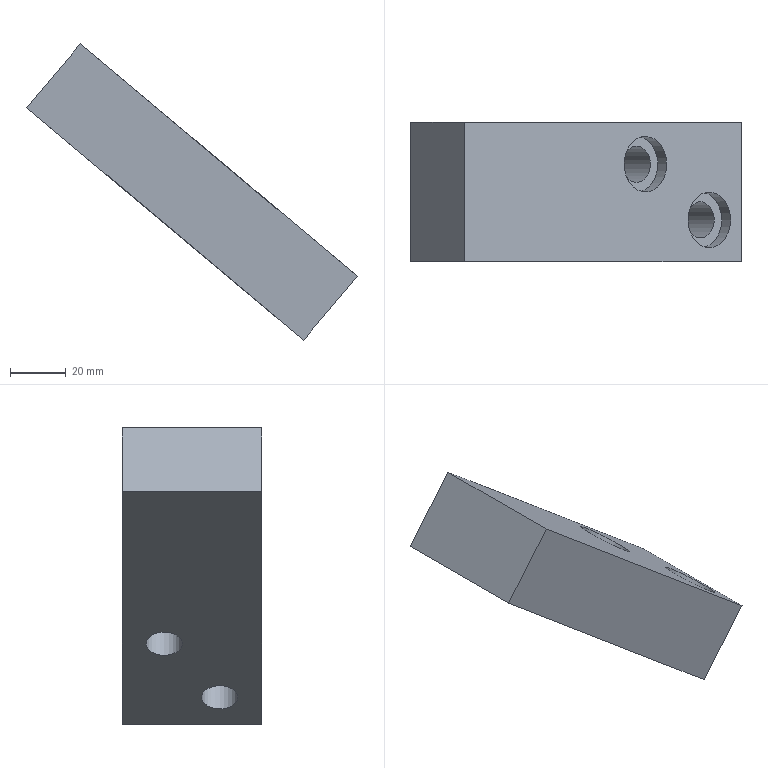Part | NX | features solid 2 | 1 solid | 12 faces | box 118.869 x 50 x 106.544 mm | volume 185222 mm3 | plane 8 | cylinder 4 | commonest cylinder face diameters 13 x2 20 x2
STEP:
#1=CARTESIAN_POINT('',(958.857,517.5,-136.861));
#2=VERTEX_POINT('',#1);
#3=CARTESIAN_POINT('',(951.197,517.5,-130.433));
#4=DIRECTION('',(-0.6428,0.,-0.766));
#5=DIRECTION('',(0.766,0.,-0.6428));
#6=AXIS2_PLACEMENT_3D('',#3,#4,#5);
#7=CIRCLE('',#6,10.);
#8=EDGE_CURVE('',#2,#2,#7,.T.);
#9=ORIENTED_EDGE('',*,*,#8,.T.);
#10=EDGE_LOOP('',(#9));
#11=FACE_BOUND('',#10,.T.);
#12=CARTESIAN_POINT('',(981.839,497.5,-156.145));
#13=VERTEX_POINT('',#12);
#14=CARTESIAN_POINT('',(974.178,497.5,-149.717));
#15=DIRECTION('',(-0.6428,0.,-0.766));
#16=DIRECTION('',(0.766,0.,-0.6428));
#17=AXIS2_PLACEMENT_3D('',#14,#15,#16);
#18=CIRCLE('',#17,10.);
#19=EDGE_CURVE('',#13,#13,#18,.T.);
#20=ORIENTED_EDGE('',*,*,#19,.T.);
#21=EDGE_LOOP('',(#20));
#22=FACE_BOUND('',#21,.T.);
#23=CARTESIAN_POINT('',(985.669,482.5,-159.359));
#24=VERTEX_POINT('',#23);
#25=CARTESIAN_POINT('',(985.669,532.5,-159.359));
#26=VERTEX_POINT('',#25);
#27=CARTESIAN_POINT('',(985.669,500.,-159.359));
#28=DIRECTION('',(0.,1.,0.));
#29=VECTOR('',#28,1000.);
#30=LINE('',#27,#29);
#31=EDGE_CURVE('',#24,#26,#30,.T.);
#32=ORIENTED_EDGE('',*,*,#31,.T.);
#33=CARTESIAN_POINT('',(886.083,532.5,-75.796));
#34=VERTEX_POINT('',#33);
#35=CARTESIAN_POINT('',(903.319,532.5,-90.259));
#36=DIRECTION('',(-0.766,0.,0.6428));
#37=VECTOR('',#36,1000.);
#38=LINE('',#35,#37);
#39=EDGE_CURVE('',#26,#34,#38,.T.);
#40=ORIENTED_EDGE('',*,*,#39,.T.);
#41=CARTESIAN_POINT('',(886.083,482.5,-75.796));
#42=VERTEX_POINT('',#41);
#43=CARTESIAN_POINT('',(886.083,500.,-75.796));
#44=DIRECTION('',(0.,-1.,0.));
#45=VECTOR('',#44,1000.);
#46=LINE('',#43,#45);
#47=EDGE_CURVE('',#34,#42,#46,.T.);
#48=ORIENTED_EDGE('',*,*,#47,.T.);
#49=CARTESIAN_POINT('',(903.319,482.5,-90.259));
#50=DIRECTION('',(0.766,0.,-0.6428));
#51=VECTOR('',#50,1000.);
#52=LINE('',#49,#51);
#53=EDGE_CURVE('',#42,#24,#52,.T.);
#54=ORIENTED_EDGE('',*,*,#53,.T.);
#55=EDGE_LOOP('',(#32,#40,#48,#54));
#56=FACE_BOUND('',#55,.T.);
#57=CARTESIAN_POINT('',(903.319,500.,-90.259));
#58=DIRECTION('',(0.6428,0.,0.766));
#59=DIRECTION('',(0.,-1.,0.));
#60=AXIS2_PLACEMENT_3D('',#57,#58,#59);
#61=PLANE('',#60);
#62=ADVANCED_FACE('',(#11,#22,#56),#61,.T.);
#63=CARTESIAN_POINT('',(966.385,482.5,-182.34));
#64=VERTEX_POINT('',#63);
#65=CARTESIAN_POINT('',(966.385,482.5,-182.34));
#66=DIRECTION('',(0.6428,0.,0.766));
#67=VECTOR('',#66,1000.);
#68=LINE('',#65,#67);
#69=EDGE_CURVE('',#64,#24,#68,.T.);
#70=ORIENTED_EDGE('',*,*,#69,.F.);
#71=CARTESIAN_POINT('',(966.385,532.5,-182.34));
#72=VERTEX_POINT('',#71);
#73=CARTESIAN_POINT('',(966.385,500.,-182.34));
#74=DIRECTION('',(0.,-1.,0.));
#75=VECTOR('',#74,1000.);
#76=LINE('',#73,#75);
#77=EDGE_CURVE('',#72,#64,#76,.T.);
#78=ORIENTED_EDGE('',*,*,#77,.F.);
#79=CARTESIAN_POINT('',(966.385,532.5,-182.34));
#80=DIRECTION('',(0.6428,0.,0.766));
#81=VECTOR('',#80,1000.);
#82=LINE('',#79,#81);
#83=EDGE_CURVE('',#72,#26,#82,.T.);
#84=ORIENTED_EDGE('',*,*,#83,.T.);
#85=ORIENTED_EDGE('',*,*,#31,.F.);
#86=EDGE_LOOP('',(#70,#78,#84,#85));
#87=FACE_BOUND('',#86,.T.);
#88=CARTESIAN_POINT('',(966.385,500.,-182.34));
#89=DIRECTION('',(0.766,0.,-0.6428));
#90=DIRECTION('',(-0.6428,0.,-0.766));
#91=AXIS2_PLACEMENT_3D('',#88,#89,#90);
#92=PLANE('',#91);
#93=ADVANCED_FACE('',(#87),#92,.T.);
#94=ORIENTED_EDGE('',*,*,#83,.F.);
#95=CARTESIAN_POINT('',(866.8,532.5,-98.778));
#96=VERTEX_POINT('',#95);
#97=CARTESIAN_POINT('',(884.036,532.5,-113.24));
#98=DIRECTION('',(0.766,0.,-0.6428));
#99=VECTOR('',#98,1000.);
#100=LINE('',#97,#99);
#101=EDGE_CURVE('',#96,#72,#100,.T.);
#102=ORIENTED_EDGE('',*,*,#101,.F.);
#103=CARTESIAN_POINT('',(866.8,532.5,-98.778));
#104=DIRECTION('',(0.6428,0.,0.766));
#105=VECTOR('',#104,1000.);
#106=LINE('',#103,#105);
#107=EDGE_CURVE('',#96,#34,#106,.T.);
#108=ORIENTED_EDGE('',*,*,#107,.T.);
#109=ORIENTED_EDGE('',*,*,#39,.F.);
#110=EDGE_LOOP('',(#94,#102,#108,#109));
#111=FACE_BOUND('',#110,.T.);
#112=CARTESIAN_POINT('',(884.036,532.5,-113.24));
#113=DIRECTION('',(0.,1.,0.));
#114=DIRECTION('',(0.6428,0.,0.766));
#115=AXIS2_PLACEMENT_3D('',#112,#113,#114);
#116=PLANE('',#115);
#117=ADVANCED_FACE('',(#111),#116,.T.);
#118=ORIENTED_EDGE('',*,*,#107,.F.);
#119=CARTESIAN_POINT('',(866.8,482.5,-98.778));
#120=VERTEX_POINT('',#119);
#121=CARTESIAN_POINT('',(866.8,500.,-98.778));
#122=DIRECTION('',(0.,1.,0.));
#123=VECTOR('',#122,1000.);
#124=LINE('',#121,#123);
#125=EDGE_CURVE('',#120,#96,#124,.T.);
#126=ORIENTED_EDGE('',*,*,#125,.F.);
#127=CARTESIAN_POINT('',(866.8,482.5,-98.778));
#128=DIRECTION('',(0.6428,0.,0.766));
#129=VECTOR('',#128,1000.);
#130=LINE('',#127,#129);
#131=EDGE_CURVE('',#120,#42,#130,.T.);
#132=ORIENTED_EDGE('',*,*,#131,.T.);
#133=ORIENTED_EDGE('',*,*,#47,.F.);
#134=EDGE_LOOP('',(#118,#126,#132,#133));
#135=FACE_BOUND('',#134,.T.);
#136=CARTESIAN_POINT('',(866.8,500.,-98.778));
#137=DIRECTION('',(-0.766,0.,0.6428));
#138=DIRECTION('',(0.6428,0.,0.766));
#139=AXIS2_PLACEMENT_3D('',#136,#137,#138);
#140=PLANE('',#139);
#141=ADVANCED_FACE('',(#135),#140,.T.);
#142=CARTESIAN_POINT('',(926.934,517.5,-149.236));
#143=VERTEX_POINT('',#142);
#144=CARTESIAN_POINT('',(931.913,517.5,-153.415));
#145=DIRECTION('',(0.6428,0.,0.766));
#146=DIRECTION('',(-0.766,0.,0.6428));
#147=AXIS2_PLACEMENT_3D('',#144,#145,#146);
#148=CIRCLE('',#147,6.5);
#149=EDGE_CURVE('',#143,#143,#148,.T.);
#150=ORIENTED_EDGE('',*,*,#149,.T.);
#151=EDGE_LOOP('',(#150));
#152=FACE_BOUND('',#151,.T.);
#153=CARTESIAN_POINT('',(949.915,497.5,-168.52));
#154=VERTEX_POINT('',#153);
#155=CARTESIAN_POINT('',(954.895,497.5,-172.698));
#156=DIRECTION('',(0.6428,0.,0.766));
#157=DIRECTION('',(-0.766,0.,0.6428));
#158=AXIS2_PLACEMENT_3D('',#155,#156,#157);
#159=CIRCLE('',#158,6.5);
#160=EDGE_CURVE('',#154,#154,#159,.T.);
#161=ORIENTED_EDGE('',*,*,#160,.T.);
#162=EDGE_LOOP('',(#161));
#163=FACE_BOUND('',#162,.T.);
#164=CARTESIAN_POINT('',(884.036,482.5,-113.24));
#165=DIRECTION('',(-0.766,0.,0.6428));
#166=VECTOR('',#165,1000.);
#167=LINE('',#164,#166);
#168=EDGE_CURVE('',#64,#120,#167,.T.);
#169=ORIENTED_EDGE('',*,*,#168,.T.);
#170=ORIENTED_EDGE('',*,*,#125,.T.);
#171=ORIENTED_EDGE('',*,*,#101,.T.);
#172=ORIENTED_EDGE('',*,*,#77,.T.);
#173=EDGE_LOOP('',(#169,#170,#171,#172));
#174=FACE_BOUND('',#173,.T.);
#175=CARTESIAN_POINT('',(884.036,500.,-113.24));
#176=DIRECTION('',(-0.6428,0.,-0.766));
#177=DIRECTION('',(0.,1.,0.));
#178=AXIS2_PLACEMENT_3D('',#175,#176,#177);
#179=PLANE('',#178);
#180=ADVANCED_FACE('',(#152,#163,#174),#179,.T.);
#181=ORIENTED_EDGE('',*,*,#168,.F.);
#182=ORIENTED_EDGE('',*,*,#69,.T.);
#183=ORIENTED_EDGE('',*,*,#53,.F.);
#184=ORIENTED_EDGE('',*,*,#131,.F.);
#185=EDGE_LOOP('',(#181,#182,#183,#184));
#186=FACE_BOUND('',#185,.T.);
#187=CARTESIAN_POINT('',(884.036,482.5,-113.24));
#188=DIRECTION('',(0.,-1.,0.));
#189=DIRECTION('',(-0.6428,0.,-0.766));
#190=AXIS2_PLACEMENT_3D('',#187,#188,#189);
#191=PLANE('',#190);
#192=ADVANCED_FACE('',(#186),#191,.T.);
#193=ORIENTED_EDGE('',*,*,#160,.F.);
#194=EDGE_LOOP('',(#193));
#195=FACE_BOUND('',#194,.T.);
#196=CARTESIAN_POINT('',(965.985,497.5,-149.369));
#197=VERTEX_POINT('',#196);
#198=CARTESIAN_POINT('',(970.964,497.5,-153.547));
#199=DIRECTION('',(0.6428,0.,0.766));
#200=DIRECTION('',(-0.766,0.,0.6428));
#201=AXIS2_PLACEMENT_3D('',#198,#199,#200);
#202=CIRCLE('',#201,6.5);
#203=EDGE_CURVE('',#197,#197,#202,.F.);
#204=ORIENTED_EDGE('',*,*,#203,.F.);
#205=EDGE_LOOP('',(#204));
#206=FACE_BOUND('',#205,.T.);
#207=CARTESIAN_POINT('',(938.825,497.5,-191.849));
#208=DIRECTION('',(0.6428,0.,0.766));
#209=DIRECTION('',(0.766,0.,-0.6428));
#210=AXIS2_PLACEMENT_3D('',#207,#208,#209);
#211=CYLINDRICAL_SURFACE('',#210,6.5);
#212=ADVANCED_FACE('',(#195,#206),#211,.F.);
#213=ORIENTED_EDGE('',*,*,#203,.T.);
#214=EDGE_LOOP('',(#213));
#215=FACE_BOUND('',#214,.T.);
#216=CARTESIAN_POINT('',(978.625,497.5,-159.975));
#217=VERTEX_POINT('',#216);
#218=CARTESIAN_POINT('',(970.964,497.5,-153.547));
#219=DIRECTION('',(-0.6428,0.,-0.766));
#220=DIRECTION('',(0.766,0.,-0.6428));
#221=AXIS2_PLACEMENT_3D('',#218,#219,#220);
#222=CIRCLE('',#221,10.);
#223=EDGE_CURVE('',#217,#217,#222,.T.);
#224=ORIENTED_EDGE('',*,*,#223,.F.);
#225=EDGE_LOOP('',(#224));
#226=FACE_BOUND('',#225,.T.);
#227=CARTESIAN_POINT('',(970.964,497.5,-153.547));
#228=DIRECTION('',(-0.6428,0.,-0.766));
#229=DIRECTION('',(-0.766,0.,0.6428));
#230=AXIS2_PLACEMENT_3D('',#227,#228,#229);
#231=PLANE('',#230);
#232=ADVANCED_FACE('',(#215,#226),#231,.F.);
#233=ORIENTED_EDGE('',*,*,#19,.F.);
#234=EDGE_LOOP('',(#233));
#235=FACE_BOUND('',#234,.T.);
#236=ORIENTED_EDGE('',*,*,#223,.T.);
#237=EDGE_LOOP('',(#236));
#238=FACE_BOUND('',#237,.T.);
#239=CARTESIAN_POINT('',(970.964,497.5,-153.547));
#240=DIRECTION('',(0.6428,0.,0.766));
#241=DIRECTION('',(0.766,0.,-0.6428));
#242=AXIS2_PLACEMENT_3D('',#239,#240,#241);
#243=CYLINDRICAL_SURFACE('',#242,10.);
#244=ADVANCED_FACE('',(#235,#238),#243,.F.);
#245=ORIENTED_EDGE('',*,*,#149,.F.);
#246=EDGE_LOOP('',(#245));
#247=FACE_BOUND('',#246,.T.);
#248=CARTESIAN_POINT('',(943.004,517.5,-130.085));
#249=VERTEX_POINT('',#248);
#250=CARTESIAN_POINT('',(947.983,517.5,-134.263));
#251=DIRECTION('',(0.6428,0.,0.766));
#252=DIRECTION('',(-0.766,0.,0.6428));
#253=AXIS2_PLACEMENT_3D('',#250,#251,#252);
#254=CIRCLE('',#253,6.5);
#255=EDGE_CURVE('',#249,#249,#254,.F.);
#256=ORIENTED_EDGE('',*,*,#255,.F.);
#257=EDGE_LOOP('',(#256));
#258=FACE_BOUND('',#257,.T.);
#259=CARTESIAN_POINT('',(915.844,517.5,-172.566));
#260=DIRECTION('',(0.6428,0.,0.766));
#261=DIRECTION('',(0.766,0.,-0.6428));
#262=AXIS2_PLACEMENT_3D('',#259,#260,#261);
#263=CYLINDRICAL_SURFACE('',#262,6.5);
#264=ADVANCED_FACE('',(#247,#258),#263,.F.);
#265=ORIENTED_EDGE('',*,*,#255,.T.);
#266=EDGE_LOOP('',(#265));
#267=FACE_BOUND('',#266,.T.);
#268=CARTESIAN_POINT('',(955.643,517.5,-140.691));
#269=VERTEX_POINT('',#268);
#270=CARTESIAN_POINT('',(947.983,517.5,-134.263));
#271=DIRECTION('',(-0.6428,0.,-0.766));
#272=DIRECTION('',(0.766,0.,-0.6428));
#273=AXIS2_PLACEMENT_3D('',#270,#271,#272);
#274=CIRCLE('',#273,10.);
#275=EDGE_CURVE('',#269,#269,#274,.T.);
#276=ORIENTED_EDGE('',*,*,#275,.F.);
#277=EDGE_LOOP('',(#276));
#278=FACE_BOUND('',#277,.T.);
#279=CARTESIAN_POINT('',(947.983,517.5,-134.263));
#280=DIRECTION('',(-0.6428,0.,-0.766));
#281=DIRECTION('',(-0.766,0.,0.6428));
#282=AXIS2_PLACEMENT_3D('',#279,#280,#281);
#283=PLANE('',#282);
#284=ADVANCED_FACE('',(#267,#278),#283,.F.);
#285=ORIENTED_EDGE('',*,*,#8,.F.);
#286=EDGE_LOOP('',(#285));
#287=FACE_BOUND('',#286,.T.);
#288=ORIENTED_EDGE('',*,*,#275,.T.);
#289=EDGE_LOOP('',(#288));
#290=FACE_BOUND('',#289,.T.);
#291=CARTESIAN_POINT('',(947.983,517.5,-134.263));
#292=DIRECTION('',(0.6428,0.,0.766));
#293=DIRECTION('',(0.766,0.,-0.6428));
#294=AXIS2_PLACEMENT_3D('',#291,#292,#293);
#295=CYLINDRICAL_SURFACE('',#294,10.);
#296=ADVANCED_FACE('',(#287,#290),#295,.F.);
#297=CLOSED_SHELL('',(#62,#93,#117,#141,#180,#192,#212,#232,#244,#264,#284,#296));
#298=MANIFOLD_SOLID_BREP('',#297);
#299=(LENGTH_UNIT()NAMED_UNIT(*)SI_UNIT(.MILLI.,.METRE.));
#300=UNCERTAINTY_MEASURE_WITH_UNIT(LENGTH_MEASURE(0.00001),#299,'','');
#301=(NAMED_UNIT(*)PLANE_ANGLE_UNIT()SI_UNIT($,.RADIAN.));
#302=(NAMED_UNIT(*)SI_UNIT($,.STERADIAN.)SOLID_ANGLE_UNIT());
#303=(GEOMETRIC_REPRESENTATION_CONTEXT(3)GLOBAL_UNCERTAINTY_ASSIGNED_CONTEXT((#300))GLOBAL_UNIT_ASSIGNED_CONTEXT((#299,#301,#302))REPRESENTATION_CONTEXT('',''));
#304=ADVANCED_BREP_SHAPE_REPRESENTATION('',(#298),#303);